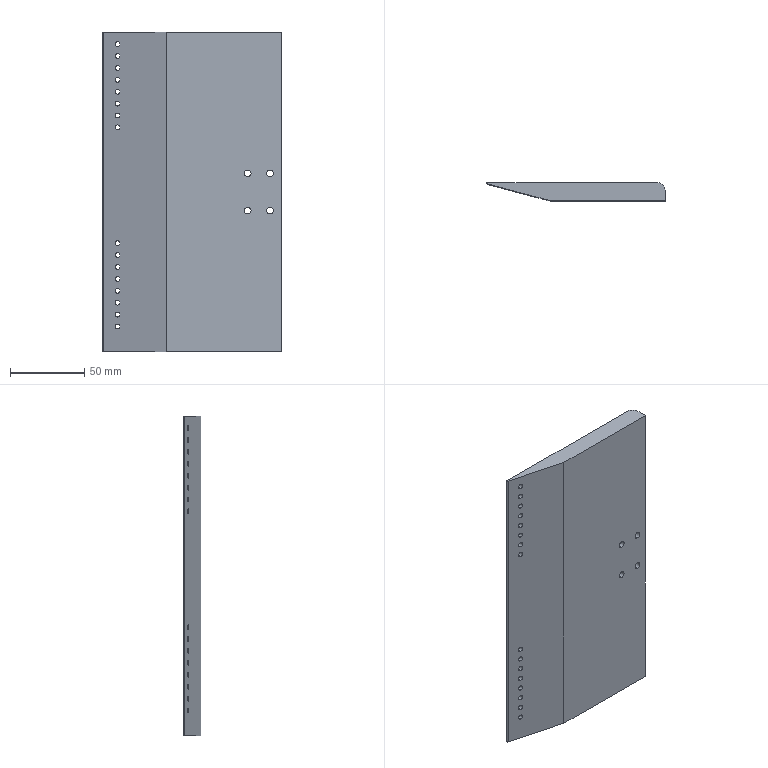Part | STEP file | MT-COMBO-119-S031 | 1 solid | 129 faces | box 120 x 12 x 215 mm | volume 252530 mm3 | cylinder 84 | cone 34 | plane 11 | commonest cylinder face diameters 3.3 x64 4.5 x8 8 x8 6 x2 1.5 x1 10 x1